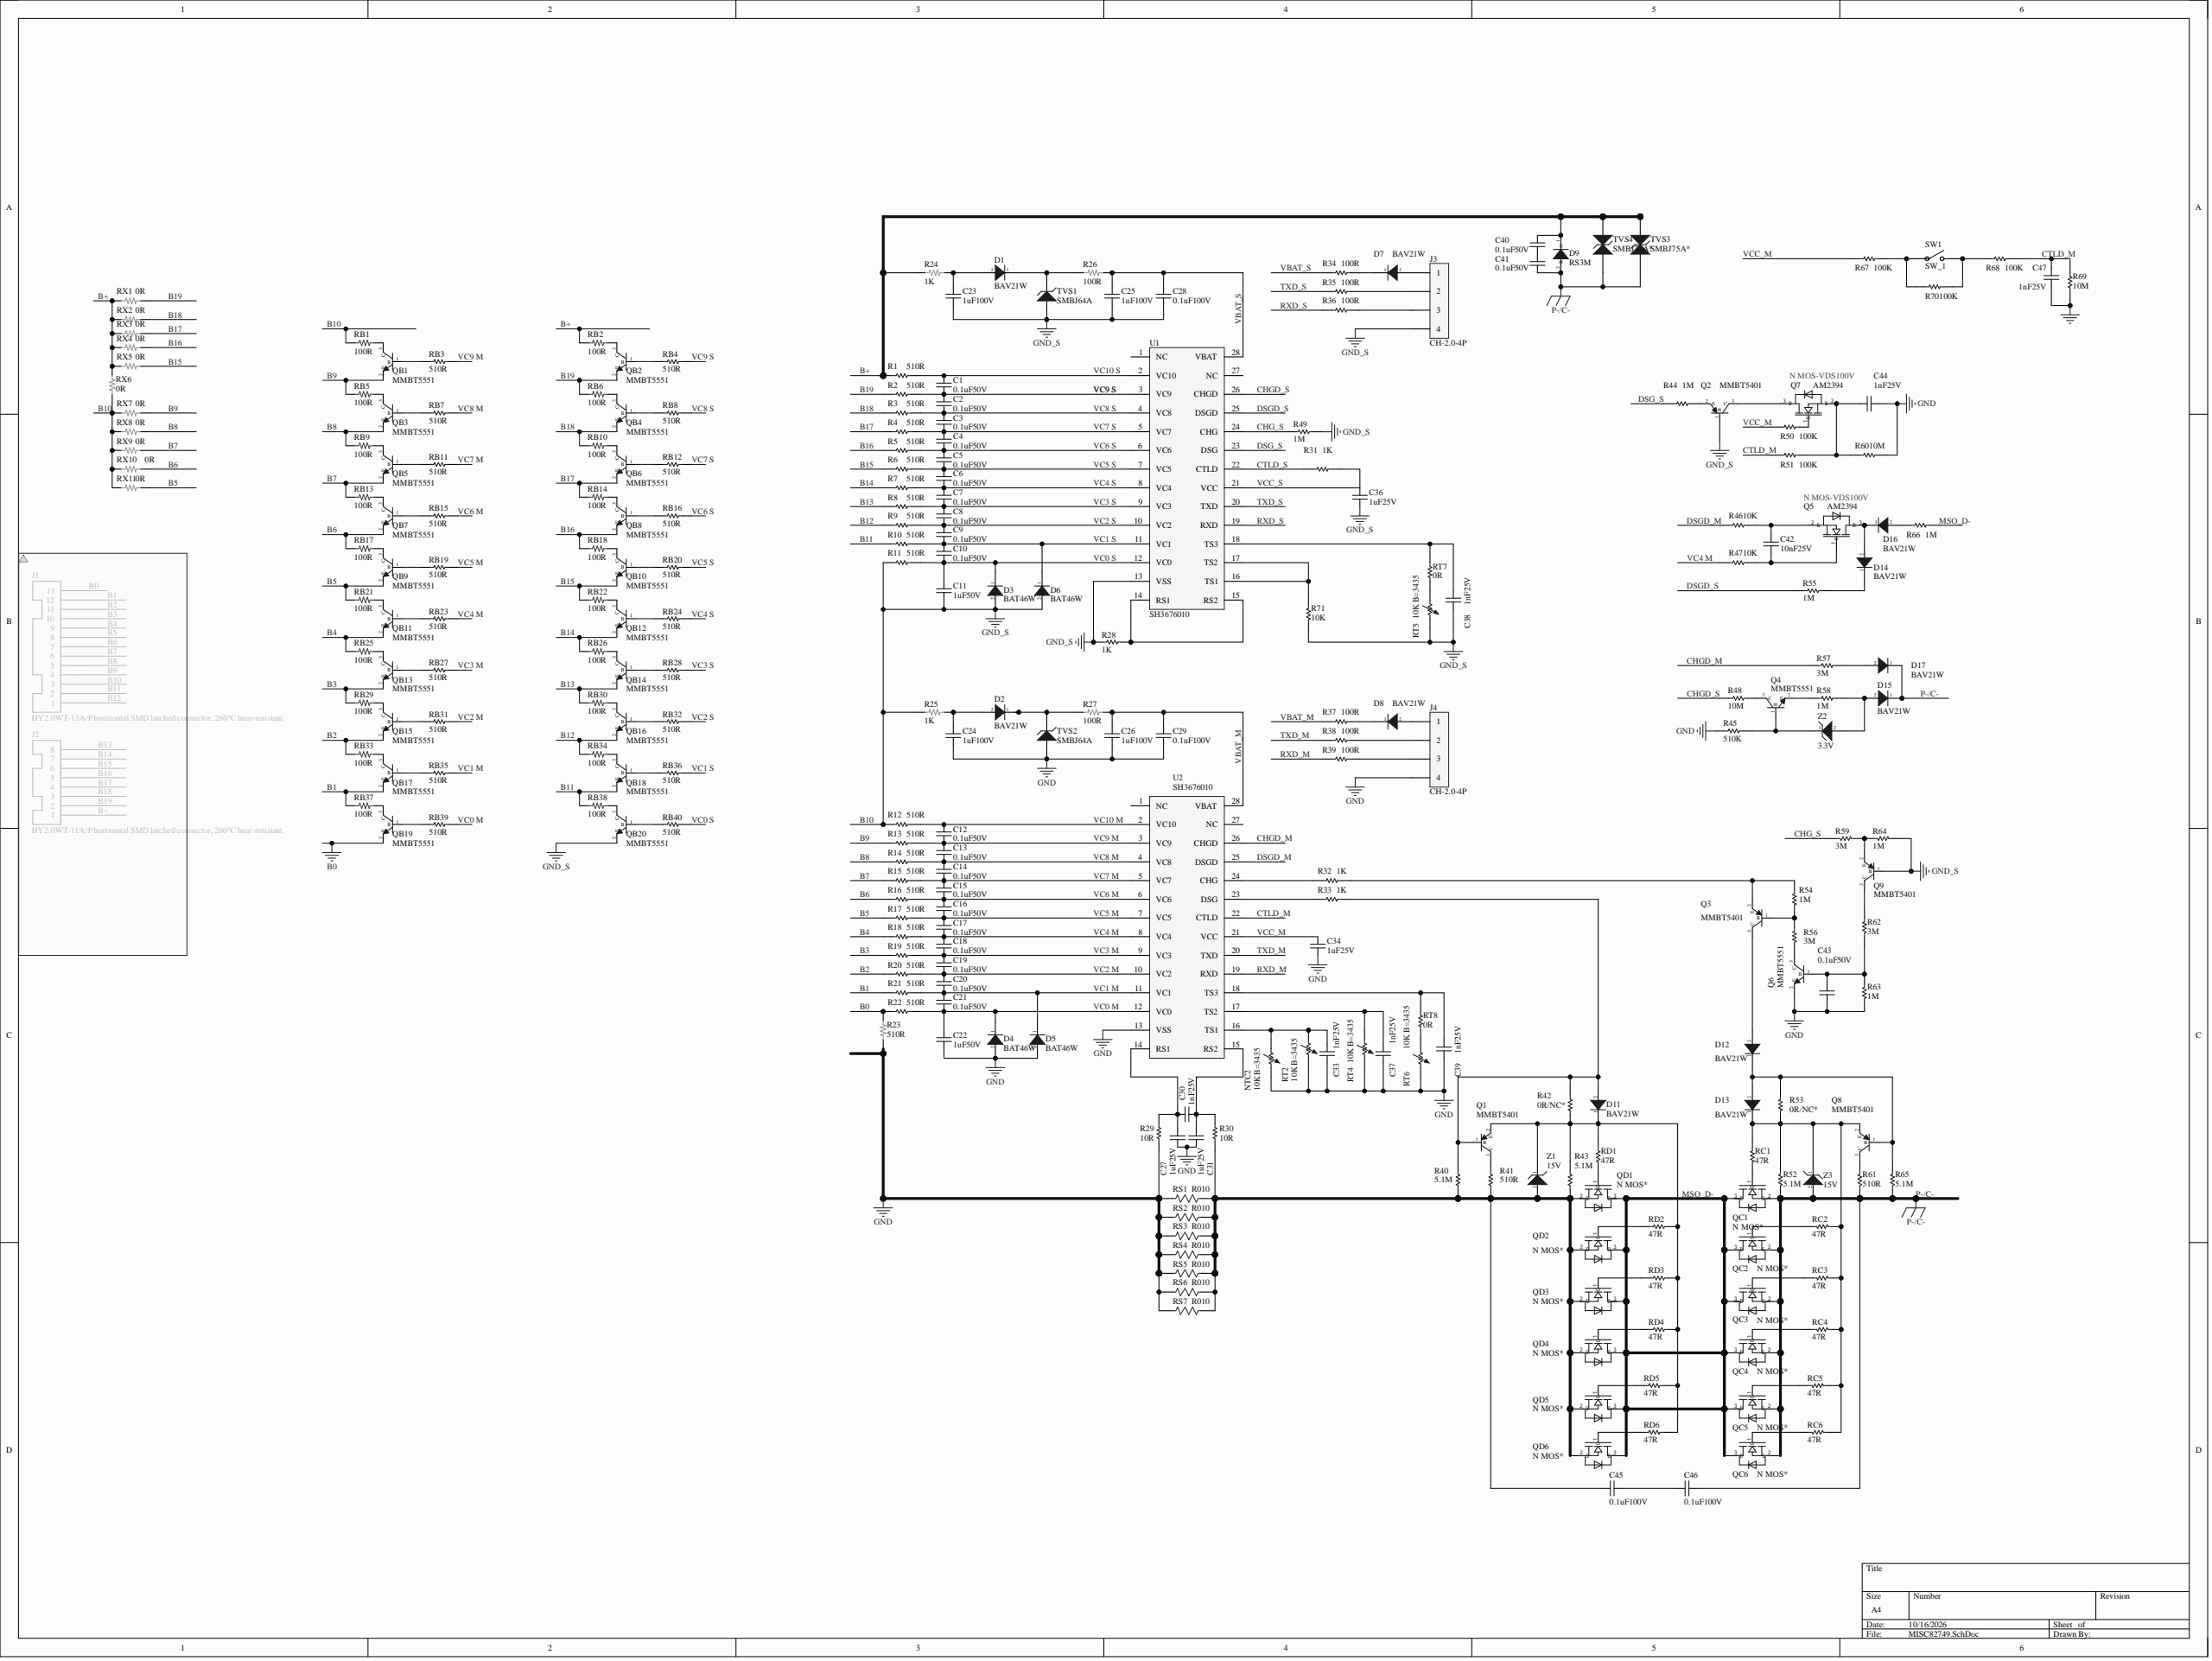Circuit board | Altium Designer | 262 parts | 170 nets
Bill of materials:
Comment,Description,Designator,Footprint,LibRef,Quantity
"0.1uF50V","SMD capacitor","C1, C2, C3, C4, C5, C6, C7, C8, C9, C10, C12, C13, C14, C15, C16, C17, C18, C19, C20, C21, C40, C41, C43","C0603A","CAP","23"
"1uF50V","SMD capacitor","C11, C22","C0603A","CAP","2"
"1uF100V","SMD capacitor","C23, C24, C25, C26","C0805L","CAP","4"
"1uF25V","SMD capacitor","C27, C31, C34, C36","C0603A","CAP","4"
"0.1uF100V","SMD capacitor","C28, C29","C0805L","CAP","2"
"1nF25V","SMD capacitor","C30, C33, C37, C38, C39, C44, C47","C0603A","CAP","7"
"10nF25V","SMD capacitor","C42","C0603A","CAP","1"
"0.1uF100V","SMD capacitor","C45, C46","C0603A","CAP","2"
"BAV21W","SMD diode","D1, D2, D7, D8, D11, D12, D13, D14, D15, D16, D17","SOD323A","BAV21_SOD323","11"
"BAT46W","SMD diode","D3, D4, D5, D6","SOD123","BAT46W_SOD123","4"
"RS3M","SMD diode","D9","SMB A","RS3M","1"
"CH-2.0-4P","test socket","J3, J4","Test2.0-4P","Test2.0-4P","2"
"10K B=3435","SMD thermistor","NTC2","RT2.3X1.2-2","NTC","1"
"MMBT5401","SMD transistor","Q1, Q2, Q3, Q8, Q9","SOT23-3","MMBT5401","5"
"MMBT5551","SMD transistor","Q4, Q6, QB1, QB2, QB3, QB4, QB5, QB6, QB7, QB8, QB9, QB10, QB11, QB12, QB13, QB14, QB15, QB16, QB17, QB18, QB19, QB20","SOT23-3","MMBT5551","22"
"AM2394","SMD N MOS_VGS100V","Q5, Q7","SOT23-3L","AM2394_VGS100V","2"
"N MOS*","SMD MOSFET","QC1, QC2, QC3, QC4, QC5, QC6, QD1, QD2, QD3, QD4, QD5, QD6","TOLL_123","N MOS*","12"
"510R","SMD resistor","R1, R2, R3, R4, R5, R6, R7, R8, R9, R10, R11, R12, R13, R14, R15, R16, R17, R18, R19, R20, R21, R22, R41, R61, RB3, RB4, RB7, RB8, RB11, RB12, RB15, RB16, RB19, RB20, RB23, RB24, RB27, RB28, RB31, RB32, RB35, RB36, RB39, RB40","R0603A","RES","44"
"510R","SMD resistor","R23","R0805L","RES_0805","1"
"1K","SMD resistor","R24, R25","R0805L","RES_0805","2"
"100R","SMD resistor","R26, R27","R0805L","RES_0805","2"
"1K","SMD resistor","R28, R31, R32, R33","R0603A","RES","4"
"10R","SMD resistor","R29, R30","R0603A","RES","2"
"100R","SMD resistor","R34, R35, R36, R37, R38, R39","R0603A","RES","6"
"5.1M","SMD resistor","R40, R43, R52, R65","R0603A","RES","4"
"0R/NC*","SMD resistor","R42, R53","R0603A","RES","2"
"1M","SMD resistor","R44, R49, R54, R55, R58, R63, R64, R66","R0603A","RES","8"
"510K","SMD resistor","R45","R0603A","RES","1"
"10K","SMD resistor","R46, R47, R71","R0603A","RES","3"
"10M","SMD resistor","R48, R60, R69","R0603A","RES","3"
"100K","SMD resistor","R50, R51, R67, R68, R70","R0603A","RES","5"
"3M","SMD resistor","R56, R57, R59, R62","R0603A","RES","4"
"100R","alloy SMD resistor","RB1, RB2, RB5, RB6, RB9, RB10, RB13, RB14, RB17, RB18, RB21, RB22, RB25, RB26, RB29, RB30, RB33, RB34, RB37, RB38","R1206A","RES3","20"
"47R","SMD resistor","RC1, RC2, RC3, RC4, RC5, RC6, RD1, RD2, RD3, RD4, RD5, RD6","R0603A","RES","12"
"R010","SMD alloy resistor","RS1, RS2, RS3, RS4, RS5, RS6, RS7","R2512L","RES2_2512","7"
"10K B=3435","SMD thermistor","RT2, RT4, RT5, RT6","R0603A","NTC","4"
"0R","SMD resistor","RT7, RT8","R0603A","RES","2"
"0R","SMD resistor","RX1, RX2, RX3, RX4, RX5, RX6, RX7, RX8, RX9, RX10, RX11","R0805L","RES_0805","11"
"SW_1","soft-touch switch","SW1","RT2.3X1.2-2","SW_1","1"
"SMBJ64A","SMD diode (ESD and surge protection)","TVS1, TVS2","SMB A","SMBJ64A","2"
"SMBJ75A*","SMD diode (ESD and surge protection)","TVS3, TVS4","SMC_MDO-214AB)","TVS C","2"
"SH3676010","","U1, U2","TSSOP-28L(PIN间距0.65mm)","SH3676010","2"
"15V","SMD zener diode","Z1, Z3","SOD323A","15V SOD323","2"
"3.3V","SMD zener diode","Z2","SOD323A","3.3_SOD323","1"
Netlist (Protel format):
[
C1
C0603A
0.1uF50V



]
[
C2
C0603A
0.1uF50V



]
[
C3
C0603A
0.1uF50V



]
[
C4
C0603A
0.1uF50V



]
[
C5
C0603A
0.1uF50V



]
[
C6
C0603A
0.1uF50V



]
[
C7
C0603A
0.1uF50V



]
[
C8
C0603A
0.1uF50V



]
[
C9
C0603A
0.1uF50V



]
[
C10
C0603A
0.1uF50V



]
[
C11
C0603A
1uF50V



]
[
C12
C0603A
0.1uF50V



]
[
C13
C0603A
0.1uF50V



]
[
C14
C0603A
0.1uF50V



]
[
C15
C0603A
0.1uF50V



]
[
C16
C0603A
0.1uF50V



]
[
C17
C0603A
0.1uF50V



]
[
C18
C0603A
0.1uF50V



]
[
C19
C0603A
0.1uF50V



]
[
C20
C0603A
0.1uF50V



]
[
C21
C0603A
0.1uF50V



]
[
C22
C0603A
1uF50V



]
[
C23
C0805L
1uF100V



]
[
C24
C0805L
1uF100V



]
[
C25
C0805L
1uF100V



]
[
C26
C0805L
1uF100V



]
[
C27
C0603A
1uF25V



]
[
C28
C0805L
0.1uF100V



]
[
C29
C0805L
0.1uF100V



]
[
C30
C0603A
1nF25V



]
[
C31
C0603A
1uF25V



]
[
C33
C0603A
1nF25V



]
[
C34
C0603A
1uF25V



]
[
C36
C0603A
1uF25V



]
[
C37
C0603A
1nF25V



]
[
C38
C0603A
1nF25V



]
[
C39
C0603A
1nF25V



]
[
C40
C0603A
0.1uF50V



]
[
C41
C0603A
0.1uF50V



]
[
C42
C0603A
10nF25V



]
[
C43
C0603A
0.1uF50V



]
[
C44
C0603A
1nF25V



]
[
C45
C0603A
0.1uF100V



]
[
C46
C0603A
0.1uF100V



]
[
C47
C0603A
1nF25V



]
[
D1
SOD323A
BAV21W



]
[
D2
SOD323A
BAV21W



]
[
D3
SOD123
BAT46W



]
[
D4
SOD123
BAT46W



]
[
D5
SOD123
BAT46W



]
[
D6
SOD123
BAT46W



]
[
D7
SOD323A
BAV21W



]
[
D8
SOD323A
BAV21W



]
[
D9
SMB A
RS3M



]
[
D11
SOD323A
BAV21W



]
[
D12
SOD323A
BAV21W



]
[
D13
SOD323A
BAV21W



]
[
D14
SOD323A
BAV21W



]
[
D15
SOD323A
BAV21W



]
[
D16
SOD323A
BAV21W



]
[
D17
SOD323A
BAV21W



]
[
J3
Test2.0-4P
CH-2.0-4P



]
[
J4
Test2.0-4P
CH-2.0-4P



]
[
NTC2
RT2.3X1.2-2
10K B=3435



]
[
Q1
SOT23-3
MMBT5401



]
[
Q2
SOT23-3
MMBT5401



]
[
Q3
SOT23-3
MMBT5401



]
[
Q4
SOT23-3
MMBT5551



]
[
Q5
SOT23-3L
AM2394



]
[
Q6
SOT23-3
MMBT5551



]
[
Q7
SOT23-3L
AM2394



]
[
Q8
SOT23-3
MMBT5401



]
[
Q9
SOT23-3
MMBT5401



]
[
QB1
SOT23-3
MMBT5551



]
[
QB2
SOT23-3
MMBT5551



]
[
QB3
SOT23-3
MMBT5551



]
[
QB4
SOT23-3
MMBT5551



]
[
QB5
SOT23-3
MMBT5551



]
[
QB6
SOT23-3
MMBT5551



]
[
QB7
SOT23-3
MMBT5551



]
[
QB8
SOT23-3
MMBT5551



]
[
QB9
SOT23-3
MMBT5551



]
[
QB10
SOT23-3
MMBT5551



]
[
QB11
SOT23-3
MMBT5551



]
[
QB12
SOT23-3
MMBT5551



]
[
QB13
SOT23-3
MMBT5551



]
[
QB14
SOT23-3
MMBT5551



]
[
QB15
SOT23-3
MMBT5551



]
[
QB16
SOT23-3
MMBT5551



]
[
QB17
SOT23-3
MMBT5551



]
[
QB18
SOT23-3
MMBT5551



]
[
QB19
SOT23-3
MMBT5551



]
[
QB20
SOT23-3
MMBT5551



]
[
QC1
TOLL_123
N MOS*



]
[
QC2
TOLL_123
N MOS*



]
[
QC3
TOLL_123
N MOS*



]
[
QC4
TOLL_123
N MOS*



]
[
QC5
TOLL_123
N MOS*



]
[
QC6
TOLL_123
N MOS*



]
[
QD1
TOLL_123
N MOS*



]
[
QD2
TOLL_123
N MOS*



]
[
QD3
TOLL_123
N MOS*



]
[
QD4
TOLL_123
N MOS*



]
[
QD5
TOLL_123
N MOS*



]
[
QD6
TOLL_123
N MOS*



]
[
R1
R0603A
510R



]
[
R2
R0603A
510R



]
[
R3
R0603A
510R



]
[
R4
R0603A
510R



]
[
R5
R0603A
510R



]
[
R6
R0603A
510R



]
[
R7
R0603A
510R



]
[
R8
R0603A
510R



]
[
R9
R0603A
510R



]
[
R10
R0603A
510R



]
[
R11
R0603A
510R



]
[
R12
R0603A
510R



]
[
R13
R0603A
510R



]
[
R14
R0603A
510R



]
[
R15
R0603A
510R



]
[
R16
R0603A
510R



]
[
R17
R0603A
510R



]
[
R18
R0603A
510R



]
[
R19
R0603A
510R



]
[
R20
R0603A
510R



]
[
R21
R0603A
510R



]
[
R22
R0603A
510R



]
[
R23
R0805L
510R



]
[
R24
R0805L
1K



]
[
R25
R0805L
1K



]
[
R26
R0805L
100R



]
[
R27
R0805L
100R



]
[
R28
R0603A
1K



]
[
R29
R0603A
10R



]
[
R30
R0603A
10R



]
[
R31
R0603A
1K



]
[
R32
R0603A
1K



]
[
R33
R0603A
1K



]
[
R34
R0603A
100R



]
[
R35
R0603A
100R



]
[
R36
R0603A
100R



]
[
R37
R0603A
100R



]
[
R38
R0603A
100R



]
[
R39
R0603A
100R



]
[
R40
R0603A
5.1M



]
[
R41
R0603A
510R



]
[
R42
R0603A
0R/NC*



]
[
R43
R0603A
5.1M



]
[
R44
R0603A
1M



]
[
R45
R0603A
510K



]
[
R46
R0603A
10K



]
[
R47
R0603A
10K



]
[
R48
R0603A
10M



]
[
R49
R0603A
1M



]
[
R50
R0603A
100K



]
[
R51
R0603A
100K



]
[
R52
R0603A
5.1M



]
[
R53
R0603A
0R/NC*



]
[
R54
R0603A
1M



]
[
R55
R0603A
1M



]
[
R56
R0603A
3M



]
[
R57
R0603A
3M



]
[
R58
R0603A
1M



]
[
R59
R0603A
3M



]
[
R60
R0603A
10M



]
[
R61
R0603A
510R



]
[
R62
R0603A
3M



]
[
R63
R0603A
1M



]
[
R64
R0603A
1M



]
[
R65
R0603A
5.1M



]
[
R66
R0603A
1M



]
[
R67
R0603A
100K



]
[
R68
R0603A
100K



]
[
R69
R0603A
10M



]
[
R70
R0603A
100K



]
[
R71
R0603A
10K



]
[
RB1
R1206A
100R



]
[
RB2
R1206A
100R



]
[
RB3
R0603A
510R



]
[
RB4
R0603A
510R



]
[
RB5
R1206A
100R



]
[
RB6
R1206A
100R



]
[
RB7
R0603A
510R



]
[
RB8
R0603A
510R



]
[
RB9
R1206A
100R



]
[
RB10
R1206A
100R



]
[
RB11
R0603A
510R



]
[
RB12
R0603A
510R



]
[
RB13
R1206A
100R



]
[
RB14
R1206A
100R



]
[
RB15
R0603A
510R



]
[
RB16
R0603A
510R



]
[
RB17
R1206A
100R



]
[
RB18
R1206A
100R



]
[
RB19
R0603A
510R



]
[
RB20
R0603A
510R



]
[
RB21
R1206A
100R



]
[
RB22
R1206A
100R



]
[
RB23
R0603A
510R



]
[
RB24
R0603A
510R



]
[
RB25
R1206A
100R



]
[
RB26
R1206A
100R



]
[
RB27
R0603A
510R



]
[
RB28
R0603A
510R



]
[
RB29
R1206A
100R



]
[
RB30
R1206A
100R



]
[
RB31
R0603A
510R



]
[
RB32
R0603A
510R



]
[
RB33
R1206A
100R



]
[
RB34
R1206A
100R



]
[
RB35
R0603A
510R



]
[
RB36
R0603A
510R



]
[
RB37
R1206A
100R



]
[
RB38
R1206A
100R



]
[
RB39
R0603A
510R



]
[
RB40
R0603A
510R



]
[
RC1
R0603A
47R



]
[
RC2
R0603A
47R



]
[
RC3
R0603A
47R



]
[
RC4
R0603A
47R



]
[
RC5
R0603A
47R



]
[
RC6
R0603A
47R



]
[
RD1
R0603A
47R



]
[
RD2
R0603A
47R



]
[
RD3
R0603A
47R



]
[
RD4
R0603A
47R



]
[
RD5
R0603A
47R



]
[
RD6
R0603A
47R



]
[
RS1
R2512L
R010



]
[
RS2
R2512L
R010



]
[
RS3
R2512L
R010



]
[
RS4
R2512L
R010



]
[
RS5
R2512L
R010



]
[
RS6
R2512L
R010



]
[
RS7
R2512L
R010



]
[
RT2
R0603A
10K B=3435



]
[
RT4
R0603A
10K B=3435



]
[
RT5
R0603A
10K B=3435



]
[
RT6
R0603A
10K B=3435



]
[
RT7
R0603A
0R



]
[
RT8
R0603A
0R



]
[
RX1
R0805L
0R



]
[
RX2
R0805L
0R



]
[
RX3
R0805L
0R



]
[
RX4
R0805L
0R



]
[
RX5
R0805L
0R



]
[
RX6
R0805L
0R



]
[
RX7
R0805L
0R



]
[
RX8
R0805L
0R



]
[
RX9
R0805L
0R



]
[
RX10
R0805L
0R



]
[
RX11
R0805L
0R



]
[
SW1
RT2.3X1.2-2
SW_1



]
[
TVS1
SMB A
SMBJ64A



]
[
TVS2
SMB A
SMBJ64A



]
[
TVS3
SMC_MDO-214AB)
SMBJ75A*



]
[
TVS4
SMC_MDO-214AB)
SMBJ75A*



]
[
U1
TSSOP-28L(PIN间距0.65mm)
SH3676010



]
[
U2
TSSOP-28L(PIN间距0.65mm)
SH3676010



]
[
Z1
SOD323A
15V



]
[
Z2
SOD323A
3.3V



]
[
Z3
SOD323A
15V



]
(
VCC_S
C36-2
R31-1
U1-21
)
(
VCC_M
C34-2
R50-2
R67-2
U2-21
)
(
VC10 S
C1-2
R1-2
U1-2
)
(
VC10 M
C12-2
R12-2
U2-2
)
(
VC9 S
C1-1
C2-2
R2-2
RB4-2
U1-3
)
(
VC9 M
C12-1
C13-2
R13-2
RB3-2
U2-3
)
(
VC8 S
C2-1
C3-2
R3-2
RB8-2
U1-4
)
(
VC8 M
C13-1
C14-2
R14-2
RB7-2
U2-4
)
(
VC7 S
C3-1
C4-2
R4-2
RB12-2
U1-5
)
(
VC7 M
C14-1
C15-2
R15-2
RB11-2
U2-5
)
(
VC6 S
C4-1
C5-2
R5-2
RB16-2
U1-6
)
(
VC6 M
C15-1
C16-2
R16-2
RB15-2
U2-6
)
(
VC5 S
C5-1
C6-2
R6-2
RB20-2
U1-7
)
(
VC5 M
C16-1
C17-2
R17-2
RB19-2
U2-7
)
(
VC4 S
C6-1
C7-2
R7-2
RB24-2
U1-8
)
(
VC4 M
C17-1
C18-2
R18-2
R47-2
RB23-2
U2-8
)
(
VC3 S
C7-1
C8-2
R8-2
RB28-2
U1-9
)
(
VC3 M
C18-1
C19-2
R19-2
RB27-2
U2-9
)
(
VC2 S
C8-1
C9-2
R9-2
RB32-2
U1-10
)
(
VC2 M
C19-1
C20-2
R20-2
RB31-2
U2-10
)
(
VC1 S
C9-1
C10-2
D6-1
R10-2
RB36-2
U1-11
)
(
VC1 M
C20-1
C21-2
D5-1
R21-2
RB35-2
U2-11
)
(
VC0 S
C10-1
C11-2
D3-1
R11-2
RB40-2
U1-12
)
(
VC0 M
C21-1
C22-2
D4-1
R22-2
RB39-2
U2-12
)
(
VBAT_S
C25-2
C28-2
R26-1
R34-1
U1-28
)
(
VBAT_M
C26-2
C29-2
R27-1
R37-1
U2-28
)
(
TXD_S
R35-1
U1-20
)
(
TXD_M
R38-1
U2-20
)
(
RXD_S
R36-1
U1-19
)
(
RXD_M
R39-1
U2-19
)
(
P-/C-
C41-1
C46-1
D9-2
D15-1
D17-1
QC1-2
QC2-2
QC3-2
QC4-2
QC5-2
QC6-2
R52-2
R61-2
R65-2
TVS3-1
TVS4-1
Z3-2
)
(
NetRT6_1
RT6-1
RT8-1
)
(
NetRT5_1
RT5-1
RT7-1
)
(
NetR71_2
R71-2
U1-16
U1-17
)
(
NetR68_2
R68-2
R70-1
SW1-2
)
(
NetR67_1
R67-1
R70-2
SW1-1
)
(
NetR33_1
R33-1
U2-23
)
(
NetR32_1
R32-1
U2-24
)
(
NetR28_2
R28-2
U1-14
U1-15
)
(
NetQD6_1
QD6-1
RD6-1
)
(
NetQD5_1
QD5-1
RD5-1
)
(
NetQD4_1
QD4-1
RD4-1
)
(
NetQD3_1
QD3-1
RD3-2
)
(
NetQD2_1
QD2-1
RD2-2
)
(
NetQD1_1
QD1-1
RD1-2
)
(
NetQC6_1
QC6-1
RC6-2
)
(
NetQC5_1
QC5-1
RC5-2
)
(
NetQC4_1
QC4-1
RC4-2
)
(
NetQC3_1
QC3-1
RC3-1
)
(
NetQC2_1
QC2-1
RC2-1
)
(
NetQC1_1
QC1-1
RC1-2
)
(
NetQB20_3
QB20-3
RB38-2
)
(
NetQB20_1
QB20-1
RB40-1
)
(
NetQB19_3
QB19-3
RB37-2
)
(
NetQB19_1
QB19-1
RB39-1
)
(
NetQB18_3
QB18-3
RB34-2
)
(
NetQB18_1
QB18-1
RB36-1
)
(
NetQB17_3
QB17-3
RB33-2
)
(
NetQB17_1
QB17-1
RB35-1
)
(
NetQB16_3
QB16-3
RB30-2
)
(
NetQB16_1
QB16-1
RB32-1
)
(
NetQB15_3
QB15-3
RB29-2
)
(
NetQB15_1
QB15-1
RB31-1
)
(
NetQB14_3
QB14-3
RB26-2
)
(
NetQB14_1
QB14-1
RB28-1
)
(
NetQB13_3
QB13-3
RB25-2
)
(
NetQB13_1
QB13-1
RB27-1
)
(
NetQB12_3
QB12-3
RB22-2
)
(
NetQB12_1
QB12-1
RB24-1
)
(
NetQB11_3
QB11-3
RB21-2
)
(
NetQB11_1
QB11-1
RB23-1
)
(
NetQB10_3
QB10-3
RB18-2
)
(
NetQB10_1
QB10-1
RB20-1
)
(
NetQB9_3
QB9-3
RB17-2
)
(
NetQB9_1
QB9-1
RB19-1
)
(
NetQB8_3
QB8-3
RB14-2
)
(
NetQB8_1
QB8-1
RB16-1
)
(
NetQB7_3
QB7-3
RB13-2
)
(
NetQB7_1
QB7-1
RB15-1
)
(
NetQB6_3
QB6-3
RB10-2
)
(
NetQB6_1
QB6-1
RB12-1
)
(
NetQB5_3
QB5-3
RB9-2
)
(
NetQB5_1
QB5-1
RB11-1
)
(
NetQB4_3
QB4-3
RB6-2
)
(
NetQB4_1
QB4-1
RB8-1
)
(
NetQB3_3
QB3-3
RB5-2
)
(
NetQB3_1
QB3-1
RB7-1
)
(
NetQB2_3
QB2-3
RB2-2
)
(
NetQB2_1
QB2-1
RB4-1
)
(
NetQB1_3
QB1-3
RB1-2
)
(
NetQB1_1
QB1-1
RB3-1
)
(
NetQ9_3
Q9-3
R62-2
)
(
NetQ9_2
Q9-2
R59-1
R64-1
)
(
NetQ8_3
Q8-3
R61-1
)
(
NetQ7_1
Q7-1
R50-1
)
(
NetQ6_3
Q6-3
R56-2
)
(
NetQ4_3
Q4-3
R48-1
)
(
NetQ4_2
Q4-2
R58-2
)
(
NetQ4_1
Q4-1
R45-2
Z2-1
)
(
NetQ3_2
Q3-2
R32-2
R54-2
)
(
NetQ3_1
Q3-1
R54-1
R56-1
)
(
NetQ2_3
Q2-3
Q7-3
)
(
NetQ2_2
Q2-2
R44-1
)
(
NetQ1_3
Q1-3
R41-1
)
(
NetJ4_3
J4-3
R39-2
)
(
NetJ4_2
J4-2
R38-2
)
(
NetJ3_3
J3-3
R36-2
)
(
NetJ3_2
J3-2
R35-2
)
(
NetD17_2
D17-2
R57-1
)
(
NetD16_2
D16-2
R66-2
)
(
NetD15_2
D15-2
R58-1
Z2-2
)
(
NetD14_2
D14-2
D16-1
Q5-3
)
(
NetD14_1
D14-1
R55-1
)
(
NetD13_1
D13-1
Q8-2
R52-1
R53-2
RC1-1
RC2-2
RC3-2
RC4-1
RC5-1
RC6-1
Z3-1
)
(
NetD12_2
D12-2
Q3-3
)
(
NetD12_1
D12-1
D13-2
Q8-1
R53-1
R65-1
)
(
NetD11_2
D11-2
Q1-1
R33-2
R40-1
R42-1
)
(
NetD11_1
D11-1
Q1-2
R42-2
R43-1
RD1-1
RD2-1
RD3-1
RD4-2
RD5-2
RD6-2
Z1-1
)
(
NetD8_2
D8-2
J4-1
)
(
NetD8_1
D8-1
R37-2
)
(
NetD7_2
D7-2
J3-1
)
(
NetD7_1
D7-1
R34-2
)
(
NetD2_1
D2-1
R27-2
TVS2-1
)
(
NetD1_1
D1-1
R26-2
TVS1-1
)
(
NetC45_2
C45-2
QD1-2
QD2-2
QD3-2
QD4-2
QD5-2
QD6-2
R30-2
R40-2
R41-2
R43-2
RS1-2
RS2-2
RS3-2
RS4-2
RS5-2
RS6-2
RS7-2
Z1-2
)
(
NetC45_1
C45-1
C46-2
)
(
NetC44_1
C44-1
Q7-2
R51-1
R60-2
)
(
NetC43_2
C43-2
Q6-1
R62-1
R63-1
)
(
NetC42_2
C42-2
Q5-2
R46-1
)
(
NetC42_1
C42-1
Q5-1
R47-1
)
(
NetC40_1
C40-1
C41-2
)
(
NetC39_1
C39-1
RT8-2
U2-18
)
(
NetC38_1
C38-1
RT7-2
U1-18
)
(
NetC37_1
C37-1
RT4-1
U2-17
)
(
NetC33_1
C33-1
NTC2-1
RT2-1
U2-16
)
(
NetC30_1
C30-1
C31-2
R30-1
U2-15
)
(
NetC27_1
C27-1
C30-2
R29-2
U2-14
)
(
NetC24_2
C24-2
D2-2
R25-1
)
(
NetC23_2
C23-2
D1-2
R24-1
)
(
MSO_D-
QC1-3
QC2-3
QC3-3
QC4-3
QC5-3
QC6-3
QD1-3
QD2-3
QD3-3
QD4-3
QD5-3
QD6-3
R66-1
)
(
GND
C22-1
C24-1
C26-1
C27-2
C29-1
C31-1
C33-2
C34-1
C37-2
C39-2
C43-1
C44-2
C47-1
D4-2
D5-2
J4-4
NTC2-2
Q6-2
R23-1
R29-1
R45-1
R60-1
R63-2
R69-2
RS1-1
RS2-1
RS3-1
RS4-1
RS5-1
RS6-1
RS7-1
RT2-2
RT4-2
RT6-2
TVS2-2
U2-13
)
(
DSGD_S
R55-2
U1-25
)
(
DSGD_M
R46-2
U2-25
)
(
DSG_S
R44-2
U1-23
)
(
CTLD_S
R31-2
U1-22
)
(
CTLD_M
C47-2
R51-2
R68-1
R69-1
U2-22
)
(
CHGD_S
R48-2
U1-26
)
(
CHGD_M
R57-2
U2-26
)
(
CHG_S
R49-1
R59-2
U1-24
)
(
B+
C40-2
D9-1
R1-1
R24-2
RB2-1
RX1-1
RX2-1
RX3-1
RX4-1
RX5-1
RX6-2
TVS3-2
TVS4-2
)
(
B19
QB2-2
R2-1
RB6-1
RX1-2
)
(
B18
QB4-2
R3-1
RB10-1
RX2-2
)
(
B17
QB6-2
R4-1
RB14-1
RX3-2
)
(
B16
QB8-2
R5-1
RB18-1
RX4-2
)
(
B15
QB10-2
R6-1
RB22-1
RX5-2
)
(
B14
QB12-2
R7-1
RB26-1
)
(
B13
QB14-2
R8-1
RB30-1
)
(
B12
QB16-2
R9-1
RB34-1
)
(
B11
QB18-2
R10-1
RB38-1
)
(
B10
C11-1
C23-1
C25-1
C28-1
C36-1
C38-2
D3-2
D6-2
J3-4
Q2-1
Q9-1
QB20-2
R11-1
R12-1
R25-2
R28-1
R49-2
R64-2
R71-1
RB1-1
RT5-2
RX6-1
RX7-1
RX8-1
RX9-1
RX10-1
RX11-1
TVS1-2
U1-13
)
(
B9
QB1-2
R13-1
RB5-1
RX7-2
)
(
B8
QB3-2
R14-1
RB9-1
RX8-2
)
(
B7
QB5-2
R15-1
RB13-1
RX9-2
)
(
B6
QB7-2
R16-1
RB17-1
RX10-2
)
(
B5
QB9-2
R17-1
RB21-1
RX11-2
)
(
B4
QB11-2
R18-1
RB25-1
)
(
B3
QB13-2
R19-1
RB29-1
)
(
B2
QB15-2
R20-1
RB33-1
)
(
B1
QB17-2
R21-1
RB37-1
)
(
B0
QB19-2
R22-1
R23-2
)